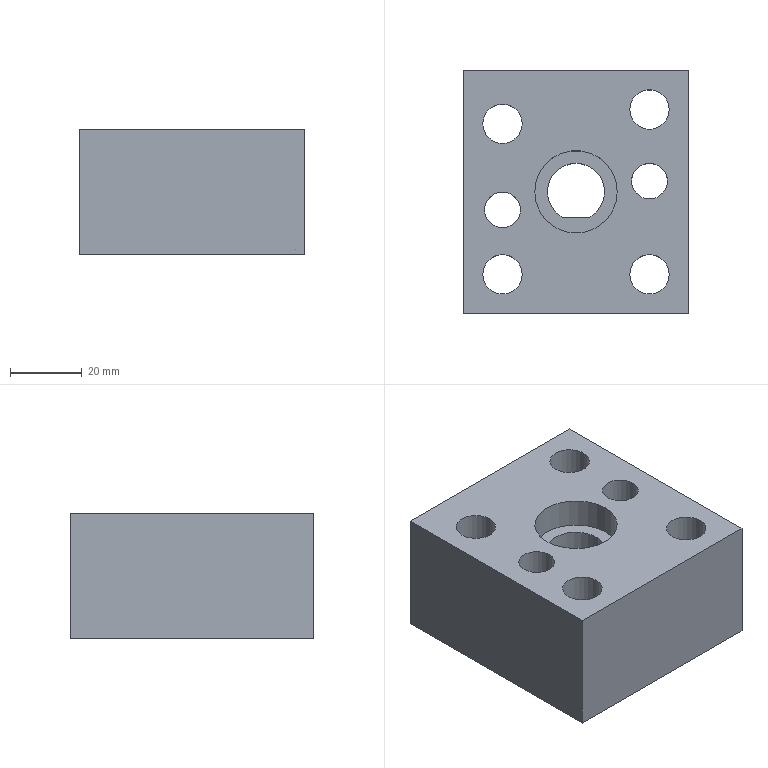Part | NX | features solid 2 | 1 solid | 28 faces | box 63 x 68 x 35 mm | volume 115819 mm3 | plane 14 | cylinder 14 | commonest cylinder face diameters 11 x6 17 x4 10 x2 16 x1 23 x1
STEP:
#1=CARTESIAN_POINT('',(1369.579,-146.904,15.));
#2=VERTEX_POINT('',#1);
#3=CARTESIAN_POINT('',(1364.579,-146.904,15.));
#4=DIRECTION('',(0.,0.,1.));
#5=DIRECTION('',(1.,0.,0.));
#6=AXIS2_PLACEMENT_3D('',#3,#4,#5);
#7=CIRCLE('',#6,5.);
#8=EDGE_CURVE('',#2,#2,#7,.T.);
#9=ORIENTED_EDGE('',*,*,#8,.T.);
#10=EDGE_LOOP('',(#9));
#11=FACE_BOUND('',#10,.T.);
#12=CARTESIAN_POINT('',(1370.079,-146.904,15.));
#13=VERTEX_POINT('',#12);
#14=CARTESIAN_POINT('',(1364.579,-146.904,15.));
#15=DIRECTION('',(0.,0.,1.));
#16=DIRECTION('',(1.,0.,0.));
#17=AXIS2_PLACEMENT_3D('',#14,#15,#16);
#18=CIRCLE('',#17,5.5);
#19=EDGE_CURVE('',#13,#13,#18,.T.);
#20=ORIENTED_EDGE('',*,*,#19,.F.);
#21=EDGE_LOOP('',(#20));
#22=FACE_BOUND('',#21,.T.);
#23=CARTESIAN_POINT('',(1363.394,-137.78,15.));
#24=DIRECTION('',(0.,0.,1.));
#25=DIRECTION('',(1.,0.,0.));
#26=AXIS2_PLACEMENT_3D('',#23,#24,#25);
#27=PLANE('',#26);
#28=ADVANCED_FACE('',(#11,#22),#27,.F.);
#29=CARTESIAN_POINT('',(1369.579,-146.904,40.));
#30=VERTEX_POINT('',#29);
#31=CARTESIAN_POINT('',(1364.579,-146.904,40.));
#32=DIRECTION('',(0.,0.,1.));
#33=DIRECTION('',(1.,0.,0.));
#34=AXIS2_PLACEMENT_3D('',#31,#32,#33);
#35=CIRCLE('',#34,5.);
#36=EDGE_CURVE('',#30,#30,#35,.T.);
#37=ORIENTED_EDGE('',*,*,#36,.T.);
#38=EDGE_LOOP('',(#37));
#39=FACE_BOUND('',#38,.T.);
#40=ORIENTED_EDGE('',*,*,#8,.F.);
#41=EDGE_LOOP('',(#40));
#42=FACE_BOUND('',#41,.T.);
#43=CARTESIAN_POINT('',(1364.579,-146.904,40.));
#44=DIRECTION('',(0.,0.,1.));
#45=DIRECTION('',(1.,0.,0.));
#46=AXIS2_PLACEMENT_3D('',#43,#44,#45);
#47=CYLINDRICAL_SURFACE('',#46,5.);
#48=ADVANCED_FACE('',(#39,#42),#47,.F.);
#49=CARTESIAN_POINT('',(1370.079,-146.904,5.));
#50=VERTEX_POINT('',#49);
#51=CARTESIAN_POINT('',(1364.579,-146.904,5.));
#52=DIRECTION('',(0.,0.,1.));
#53=DIRECTION('',(1.,0.,0.));
#54=AXIS2_PLACEMENT_3D('',#51,#52,#53);
#55=CIRCLE('',#54,5.5);
#56=EDGE_CURVE('',#50,#50,#55,.F.);
#57=ORIENTED_EDGE('',*,*,#56,.T.);
#58=EDGE_LOOP('',(#57));
#59=FACE_BOUND('',#58,.T.);
#60=ORIENTED_EDGE('',*,*,#19,.T.);
#61=EDGE_LOOP('',(#60));
#62=FACE_BOUND('',#61,.T.);
#63=CARTESIAN_POINT('',(1364.579,-146.904,5.));
#64=DIRECTION('',(0.,0.,1.));
#65=DIRECTION('',(1.,0.,0.));
#66=AXIS2_PLACEMENT_3D('',#63,#64,#65);
#67=CYLINDRICAL_SURFACE('',#66,5.5);
#68=ADVANCED_FACE('',(#59,#62),#67,.F.);
#69=CARTESIAN_POINT('',(1400.079,-164.904,17.));
#70=VERTEX_POINT('',#69);
#71=CARTESIAN_POINT('',(1405.579,-164.904,17.));
#72=DIRECTION('',(0.,0.,1.));
#73=DIRECTION('',(-1.,0.,0.));
#74=AXIS2_PLACEMENT_3D('',#71,#72,#73);
#75=CIRCLE('',#74,5.5);
#76=EDGE_CURVE('',#70,#70,#75,.T.);
#77=ORIENTED_EDGE('',*,*,#76,.T.);
#78=EDGE_LOOP('',(#77));
#79=FACE_BOUND('',#78,.T.);
#80=CARTESIAN_POINT('',(1397.079,-164.904,17.));
#81=VERTEX_POINT('',#80);
#82=CARTESIAN_POINT('',(1405.579,-164.904,17.));
#83=DIRECTION('',(0.,0.,1.));
#84=DIRECTION('',(-1.,0.,0.));
#85=AXIS2_PLACEMENT_3D('',#82,#83,#84);
#86=CIRCLE('',#85,8.5);
#87=EDGE_CURVE('',#81,#81,#86,.T.);
#88=ORIENTED_EDGE('',*,*,#87,.F.);
#89=EDGE_LOOP('',(#88));
#90=FACE_BOUND('',#89,.T.);
#91=CARTESIAN_POINT('',(1405.574,-163.238,17.));
#92=DIRECTION('',(0.,0.,1.));
#93=DIRECTION('',(-1.,0.,0.));
#94=AXIS2_PLACEMENT_3D('',#91,#92,#93);
#95=PLANE('',#94);
#96=ADVANCED_FACE('',(#79,#90),#95,.F.);
#97=CARTESIAN_POINT('',(1370.079,-164.904,17.));
#98=VERTEX_POINT('',#97);
#99=CARTESIAN_POINT('',(1364.579,-164.904,17.));
#100=DIRECTION('',(0.,0.,-1.));
#101=DIRECTION('',(1.,0.,0.));
#102=AXIS2_PLACEMENT_3D('',#99,#100,#101);
#103=CIRCLE('',#102,5.5);
#104=EDGE_CURVE('',#98,#98,#103,.F.);
#105=ORIENTED_EDGE('',*,*,#104,.T.);
#106=EDGE_LOOP('',(#105));
#107=FACE_BOUND('',#106,.T.);
#108=CARTESIAN_POINT('',(1373.079,-164.904,17.));
#109=VERTEX_POINT('',#108);
#110=CARTESIAN_POINT('',(1364.579,-164.904,17.));
#111=DIRECTION('',(0.,0.,-1.));
#112=DIRECTION('',(1.,0.,0.));
#113=AXIS2_PLACEMENT_3D('',#110,#111,#112);
#114=CIRCLE('',#113,8.5);
#115=EDGE_CURVE('',#109,#109,#114,.F.);
#116=ORIENTED_EDGE('',*,*,#115,.F.);
#117=EDGE_LOOP('',(#116));
#118=FACE_BOUND('',#117,.T.);
#119=CARTESIAN_POINT('',(1364.583,-163.238,17.));
#120=DIRECTION('',(0.,0.,1.));
#121=DIRECTION('',(1.,0.,0.));
#122=AXIS2_PLACEMENT_3D('',#119,#120,#121);
#123=PLANE('',#122);
#124=ADVANCED_FACE('',(#107,#118),#123,.F.);
#125=CARTESIAN_POINT('',(1416.579,-107.904,5.));
#126=VERTEX_POINT('',#125);
#127=CARTESIAN_POINT('',(1416.579,-175.904,5.));
#128=VERTEX_POINT('',#127);
#129=CARTESIAN_POINT('',(1416.579,-141.904,5.));
#130=DIRECTION('',(0.,-1.,0.));
#131=VECTOR('',#130,1000.);
#132=LINE('',#129,#131);
#133=EDGE_CURVE('',#126,#128,#132,.T.);
#134=ORIENTED_EDGE('',*,*,#133,.F.);
#135=CARTESIAN_POINT('',(1416.579,-107.904,40.));
#136=VERTEX_POINT('',#135);
#137=CARTESIAN_POINT('',(1416.579,-107.904,12.));
#138=DIRECTION('',(0.,0.,1.));
#139=VECTOR('',#138,1000.);
#140=LINE('',#137,#139);
#141=EDGE_CURVE('',#126,#136,#140,.T.);
#142=ORIENTED_EDGE('',*,*,#141,.T.);
#143=CARTESIAN_POINT('',(1416.579,-175.904,40.));
#144=VERTEX_POINT('',#143);
#145=CARTESIAN_POINT('',(1416.579,-141.904,40.));
#146=DIRECTION('',(0.,-1.,0.));
#147=VECTOR('',#146,1000.);
#148=LINE('',#145,#147);
#149=EDGE_CURVE('',#144,#136,#148,.F.);
#150=ORIENTED_EDGE('',*,*,#149,.F.);
#151=CARTESIAN_POINT('',(1416.579,-175.904,12.));
#152=DIRECTION('',(0.,0.,1.));
#153=VECTOR('',#152,1000.);
#154=LINE('',#151,#153);
#155=EDGE_CURVE('',#128,#144,#154,.T.);
#156=ORIENTED_EDGE('',*,*,#155,.F.);
#157=EDGE_LOOP('',(#134,#142,#150,#156));
#158=FACE_BOUND('',#157,.T.);
#159=CARTESIAN_POINT('',(1416.579,-141.904,12.));
#160=DIRECTION('',(1.,0.,0.));
#161=DIRECTION('',(0.,0.,1.));
#162=AXIS2_PLACEMENT_3D('',#159,#160,#161);
#163=PLANE('',#162);
#164=ADVANCED_FACE('',(#158),#163,.T.);
#165=CARTESIAN_POINT('',(1353.579,-107.904,40.));
#166=VERTEX_POINT('',#165);
#167=CARTESIAN_POINT('',(1353.579,-175.904,40.));
#168=VERTEX_POINT('',#167);
#169=CARTESIAN_POINT('',(1353.579,-141.904,40.));
#170=DIRECTION('',(0.,1.,0.));
#171=VECTOR('',#170,1000.);
#172=LINE('',#169,#171);
#173=EDGE_CURVE('',#166,#168,#172,.F.);
#174=ORIENTED_EDGE('',*,*,#173,.F.);
#175=CARTESIAN_POINT('',(1353.579,-107.904,5.));
#176=VERTEX_POINT('',#175);
#177=CARTESIAN_POINT('',(1353.579,-107.904,12.));
#178=DIRECTION('',(0.,0.,1.));
#179=VECTOR('',#178,1000.);
#180=LINE('',#177,#179);
#181=EDGE_CURVE('',#176,#166,#180,.T.);
#182=ORIENTED_EDGE('',*,*,#181,.F.);
#183=CARTESIAN_POINT('',(1353.579,-175.904,5.));
#184=VERTEX_POINT('',#183);
#185=CARTESIAN_POINT('',(1353.579,-141.904,5.));
#186=DIRECTION('',(0.,1.,0.));
#187=VECTOR('',#186,1000.);
#188=LINE('',#185,#187);
#189=EDGE_CURVE('',#184,#176,#188,.T.);
#190=ORIENTED_EDGE('',*,*,#189,.F.);
#191=CARTESIAN_POINT('',(1353.579,-175.904,12.));
#192=DIRECTION('',(0.,0.,1.));
#193=VECTOR('',#192,1000.);
#194=LINE('',#191,#193);
#195=EDGE_CURVE('',#184,#168,#194,.T.);
#196=ORIENTED_EDGE('',*,*,#195,.T.);
#197=EDGE_LOOP('',(#174,#182,#190,#196));
#198=FACE_BOUND('',#197,.T.);
#199=CARTESIAN_POINT('',(1353.579,-141.904,12.));
#200=DIRECTION('',(-1.,0.,0.));
#201=DIRECTION('',(0.,0.,-1.));
#202=AXIS2_PLACEMENT_3D('',#199,#200,#201);
#203=PLANE('',#202);
#204=ADVANCED_FACE('',(#198),#203,.T.);
#205=ORIENTED_EDGE('',*,*,#195,.F.);
#206=CARTESIAN_POINT('',(1385.079,-175.904,5.));
#207=DIRECTION('',(-1.,0.,0.));
#208=VECTOR('',#207,1000.);
#209=LINE('',#206,#208);
#210=EDGE_CURVE('',#128,#184,#209,.T.);
#211=ORIENTED_EDGE('',*,*,#210,.F.);
#212=ORIENTED_EDGE('',*,*,#155,.T.);
#213=CARTESIAN_POINT('',(1385.079,-175.904,40.));
#214=DIRECTION('',(-1.,0.,0.));
#215=VECTOR('',#214,1000.);
#216=LINE('',#213,#215);
#217=EDGE_CURVE('',#168,#144,#216,.F.);
#218=ORIENTED_EDGE('',*,*,#217,.F.);
#219=EDGE_LOOP('',(#205,#211,#212,#218));
#220=FACE_BOUND('',#219,.T.);
#221=CARTESIAN_POINT('',(1385.079,-175.904,12.));
#222=DIRECTION('',(0.,-1.,0.));
#223=DIRECTION('',(0.,0.,-1.));
#224=AXIS2_PLACEMENT_3D('',#221,#222,#223);
#225=PLANE('',#224);
#226=ADVANCED_FACE('',(#220),#225,.T.);
#227=CARTESIAN_POINT('',(1400.079,-164.904,40.));
#228=VERTEX_POINT('',#227);
#229=CARTESIAN_POINT('',(1405.579,-164.904,40.));
#230=DIRECTION('',(0.,0.,1.));
#231=DIRECTION('',(-1.,0.,0.));
#232=AXIS2_PLACEMENT_3D('',#229,#230,#231);
#233=CIRCLE('',#232,5.5);
#234=EDGE_CURVE('',#228,#228,#233,.T.);
#235=ORIENTED_EDGE('',*,*,#234,.T.);
#236=EDGE_LOOP('',(#235));
#237=FACE_BOUND('',#236,.T.);
#238=ORIENTED_EDGE('',*,*,#76,.F.);
#239=EDGE_LOOP('',(#238));
#240=FACE_BOUND('',#239,.T.);
#241=CARTESIAN_POINT('',(1405.579,-164.904,40.));
#242=DIRECTION('',(0.,0.,1.));
#243=DIRECTION('',(-1.,0.,0.));
#244=AXIS2_PLACEMENT_3D('',#241,#242,#243);
#245=CYLINDRICAL_SURFACE('',#244,5.5);
#246=ADVANCED_FACE('',(#237,#240),#245,.F.);
#247=CARTESIAN_POINT('',(1370.079,-164.904,40.));
#248=VERTEX_POINT('',#247);
#249=CARTESIAN_POINT('',(1364.579,-164.904,40.));
#250=DIRECTION('',(0.,0.,-1.));
#251=DIRECTION('',(1.,0.,0.));
#252=AXIS2_PLACEMENT_3D('',#249,#250,#251);
#253=CIRCLE('',#252,5.5);
#254=EDGE_CURVE('',#248,#248,#253,.F.);
#255=ORIENTED_EDGE('',*,*,#254,.T.);
#256=EDGE_LOOP('',(#255));
#257=FACE_BOUND('',#256,.T.);
#258=ORIENTED_EDGE('',*,*,#104,.F.);
#259=EDGE_LOOP('',(#258));
#260=FACE_BOUND('',#259,.T.);
#261=CARTESIAN_POINT('',(1364.579,-164.904,40.));
#262=DIRECTION('',(0.,0.,1.));
#263=DIRECTION('',(1.,0.,0.));
#264=AXIS2_PLACEMENT_3D('',#261,#262,#263);
#265=CYLINDRICAL_SURFACE('',#264,5.5);
#266=ADVANCED_FACE('',(#257,#260),#265,.F.);
#267=ORIENTED_EDGE('',*,*,#36,.F.);
#268=EDGE_LOOP('',(#267));
#269=FACE_BOUND('',#268,.T.);
#270=ORIENTED_EDGE('',*,*,#149,.T.);
#271=CARTESIAN_POINT('',(1385.079,-107.904,40.));
#272=DIRECTION('',(1.,0.,0.));
#273=VECTOR('',#272,1000.);
#274=LINE('',#271,#273);
#275=EDGE_CURVE('',#136,#166,#274,.F.);
#276=ORIENTED_EDGE('',*,*,#275,.T.);
#277=ORIENTED_EDGE('',*,*,#173,.T.);
#278=ORIENTED_EDGE('',*,*,#217,.T.);
#279=EDGE_LOOP('',(#270,#276,#277,#278));
#280=FACE_BOUND('',#279,.T.);
#281=CARTESIAN_POINT('',(1373.579,-141.904,40.));
#282=VERTEX_POINT('',#281);
#283=CARTESIAN_POINT('',(1385.079,-141.904,40.));
#284=DIRECTION('',(0.,0.,-1.));
#285=DIRECTION('',(-1.,0.,0.));
#286=AXIS2_PLACEMENT_3D('',#283,#284,#285);
#287=CIRCLE('',#286,11.5);
#288=EDGE_CURVE('',#282,#282,#287,.F.);
#289=ORIENTED_EDGE('',*,*,#288,.F.);
#290=EDGE_LOOP('',(#289));
#291=FACE_BOUND('',#290,.T.);
#292=ORIENTED_EDGE('',*,*,#254,.F.);
#293=EDGE_LOOP('',(#292));
#294=FACE_BOUND('',#293,.T.);
#295=ORIENTED_EDGE('',*,*,#234,.F.);
#296=EDGE_LOOP('',(#295));
#297=FACE_BOUND('',#296,.T.);
#298=CARTESIAN_POINT('',(1400.079,-118.904,40.));
#299=VERTEX_POINT('',#298);
#300=CARTESIAN_POINT('',(1405.579,-118.904,40.));
#301=DIRECTION('',(0.,0.,-1.));
#302=DIRECTION('',(-1.,0.,0.));
#303=AXIS2_PLACEMENT_3D('',#300,#301,#302);
#304=CIRCLE('',#303,5.5);
#305=EDGE_CURVE('',#299,#299,#304,.T.);
#306=ORIENTED_EDGE('',*,*,#305,.T.);
#307=EDGE_LOOP('',(#306));
#308=FACE_BOUND('',#307,.T.);
#309=CARTESIAN_POINT('',(1370.079,-122.904,40.));
#310=VERTEX_POINT('',#309);
#311=CARTESIAN_POINT('',(1364.579,-122.904,40.));
#312=DIRECTION('',(0.,0.,1.));
#313=DIRECTION('',(1.,0.,0.));
#314=AXIS2_PLACEMENT_3D('',#311,#312,#313);
#315=CIRCLE('',#314,5.5);
#316=EDGE_CURVE('',#310,#310,#315,.T.);
#317=ORIENTED_EDGE('',*,*,#316,.F.);
#318=EDGE_LOOP('',(#317));
#319=FACE_BOUND('',#318,.T.);
#320=CARTESIAN_POINT('',(1400.579,-138.904,40.));
#321=VERTEX_POINT('',#320);
#322=CARTESIAN_POINT('',(1405.579,-138.904,40.));
#323=DIRECTION('',(0.,0.,-1.));
#324=DIRECTION('',(-1.,0.,0.));
#325=AXIS2_PLACEMENT_3D('',#322,#323,#324);
#326=CIRCLE('',#325,5.);
#327=EDGE_CURVE('',#321,#321,#326,.T.);
#328=ORIENTED_EDGE('',*,*,#327,.T.);
#329=EDGE_LOOP('',(#328));
#330=FACE_BOUND('',#329,.T.);
#331=CARTESIAN_POINT('',(2186.158,-0.000000688,40.));
#332=DIRECTION('',(0.,0.,-1.));
#333=DIRECTION('',(1.,0.,0.));
#334=AXIS2_PLACEMENT_3D('',#331,#332,#333);
#335=PLANE('',#334);
#336=ADVANCED_FACE('',(#269,#280,#291,#294,#297,#308,#319,#330),#335,.F.);
#337=ORIENTED_EDGE('',*,*,#87,.T.);
#338=EDGE_LOOP('',(#337));
#339=FACE_BOUND('',#338,.T.);
#340=CARTESIAN_POINT('',(1397.079,-164.904,5.));
#341=VERTEX_POINT('',#340);
#342=CARTESIAN_POINT('',(1405.579,-164.904,5.));
#343=DIRECTION('',(0.,0.,1.));
#344=DIRECTION('',(-1.,0.,0.));
#345=AXIS2_PLACEMENT_3D('',#342,#343,#344);
#346=CIRCLE('',#345,8.5);
#347=EDGE_CURVE('',#341,#341,#346,.F.);
#348=ORIENTED_EDGE('',*,*,#347,.T.);
#349=EDGE_LOOP('',(#348));
#350=FACE_BOUND('',#349,.T.);
#351=CARTESIAN_POINT('',(1405.579,-164.904,5.));
#352=DIRECTION('',(0.,0.,1.));
#353=DIRECTION('',(-1.,0.,0.));
#354=AXIS2_PLACEMENT_3D('',#351,#352,#353);
#355=CYLINDRICAL_SURFACE('',#354,8.5);
#356=ADVANCED_FACE('',(#339,#350),#355,.F.);
#357=ORIENTED_EDGE('',*,*,#115,.T.);
#358=EDGE_LOOP('',(#357));
#359=FACE_BOUND('',#358,.T.);
#360=CARTESIAN_POINT('',(1373.079,-164.904,5.));
#361=VERTEX_POINT('',#360);
#362=CARTESIAN_POINT('',(1364.579,-164.904,5.));
#363=DIRECTION('',(0.,0.,-1.));
#364=DIRECTION('',(1.,0.,0.));
#365=AXIS2_PLACEMENT_3D('',#362,#363,#364);
#366=CIRCLE('',#365,8.5);
#367=EDGE_CURVE('',#361,#361,#366,.T.);
#368=ORIENTED_EDGE('',*,*,#367,.T.);
#369=EDGE_LOOP('',(#368));
#370=FACE_BOUND('',#369,.T.);
#371=CARTESIAN_POINT('',(1364.579,-164.904,5.));
#372=DIRECTION('',(0.,0.,1.));
#373=DIRECTION('',(1.,0.,0.));
#374=AXIS2_PLACEMENT_3D('',#371,#372,#373);
#375=CYLINDRICAL_SURFACE('',#374,8.5);
#376=ADVANCED_FACE('',(#359,#370),#375,.F.);
#377=CARTESIAN_POINT('',(1388.952,-148.904,5.));
#378=VERTEX_POINT('',#377);
#379=CARTESIAN_POINT('',(1381.206,-148.904,5.));
#380=VERTEX_POINT('',#379);
#381=CARTESIAN_POINT('',(1385.079,-148.904,5.));
#382=DIRECTION('',(-1.,0.,0.));
#383=VECTOR('',#382,1000.);
#384=LINE('',#381,#383);
#385=EDGE_CURVE('',#378,#380,#384,.T.);
#386=ORIENTED_EDGE('',*,*,#385,.F.);
#387=CARTESIAN_POINT('',(1385.079,-141.904,5.));
#388=DIRECTION('',(0.,0.,-1.));
#389=DIRECTION('',(-1.,0.,0.));
#390=AXIS2_PLACEMENT_3D('',#387,#388,#389);
#391=CIRCLE('',#390,8.);
#392=EDGE_CURVE('',#378,#380,#391,.F.);
#393=ORIENTED_EDGE('',*,*,#392,.T.);
#394=EDGE_LOOP('',(#386,#393));
#395=FACE_BOUND('',#394,.T.);
#396=CARTESIAN_POINT('',(1385.079,-107.904,5.));
#397=DIRECTION('',(1.,0.,0.));
#398=VECTOR('',#397,1000.);
#399=LINE('',#396,#398);
#400=EDGE_CURVE('',#176,#126,#399,.T.);
#401=ORIENTED_EDGE('',*,*,#400,.T.);
#402=ORIENTED_EDGE('',*,*,#133,.T.);
#403=ORIENTED_EDGE('',*,*,#210,.T.);
#404=ORIENTED_EDGE('',*,*,#189,.T.);
#405=EDGE_LOOP('',(#401,#402,#403,#404));
#406=FACE_BOUND('',#405,.T.);
#407=ORIENTED_EDGE('',*,*,#56,.F.);
#408=EDGE_LOOP('',(#407));
#409=FACE_BOUND('',#408,.T.);
#410=ORIENTED_EDGE('',*,*,#367,.F.);
#411=EDGE_LOOP('',(#410));
#412=FACE_BOUND('',#411,.T.);
#413=ORIENTED_EDGE('',*,*,#347,.F.);
#414=EDGE_LOOP('',(#413));
#415=FACE_BOUND('',#414,.T.);
#416=CARTESIAN_POINT('',(1397.079,-118.904,5.));
#417=VERTEX_POINT('',#416);
#418=CARTESIAN_POINT('',(1405.579,-118.904,5.));
#419=DIRECTION('',(0.,0.,-1.));
#420=DIRECTION('',(-1.,0.,0.));
#421=AXIS2_PLACEMENT_3D('',#418,#419,#420);
#422=CIRCLE('',#421,8.5);
#423=EDGE_CURVE('',#417,#417,#422,.T.);
#424=ORIENTED_EDGE('',*,*,#423,.F.);
#425=EDGE_LOOP('',(#424));
#426=FACE_BOUND('',#425,.T.);
#427=CARTESIAN_POINT('',(1373.079,-122.904,5.));
#428=VERTEX_POINT('',#427);
#429=CARTESIAN_POINT('',(1364.579,-122.904,5.));
#430=DIRECTION('',(0.,0.,1.));
#431=DIRECTION('',(1.,0.,0.));
#432=AXIS2_PLACEMENT_3D('',#429,#430,#431);
#433=CIRCLE('',#432,8.5);
#434=EDGE_CURVE('',#428,#428,#433,.F.);
#435=ORIENTED_EDGE('',*,*,#434,.F.);
#436=EDGE_LOOP('',(#435));
#437=FACE_BOUND('',#436,.T.);
#438=CARTESIAN_POINT('',(1400.079,-138.904,5.));
#439=VERTEX_POINT('',#438);
#440=CARTESIAN_POINT('',(1405.579,-138.904,5.));
#441=DIRECTION('',(0.,0.,-1.));
#442=DIRECTION('',(-1.,0.,0.));
#443=AXIS2_PLACEMENT_3D('',#440,#441,#442);
#444=CIRCLE('',#443,5.5);
#445=EDGE_CURVE('',#439,#439,#444,.T.);
#446=ORIENTED_EDGE('',*,*,#445,.F.);
#447=EDGE_LOOP('',(#446));
#448=FACE_BOUND('',#447,.T.);
#449=CARTESIAN_POINT('',(1385.079,-141.904,5.));
#450=DIRECTION('',(0.,0.,-1.));
#451=DIRECTION('',(1.,0.,0.));
#452=AXIS2_PLACEMENT_3D('',#449,#450,#451);
#453=PLANE('',#452);
#454=ADVANCED_FACE('',(#395,#406,#409,#412,#415,#426,#437,#448),#453,.T.);
#455=CARTESIAN_POINT('',(1373.579,-141.904,31.8));
#456=VERTEX_POINT('',#455);
#457=CARTESIAN_POINT('',(1385.079,-141.904,31.8));
#458=DIRECTION('',(0.,0.,-1.));
#459=DIRECTION('',(-1.,0.,0.));
#460=AXIS2_PLACEMENT_3D('',#457,#458,#459);
#461=CIRCLE('',#460,11.5);
#462=EDGE_CURVE('',#456,#456,#461,.T.);
#463=ORIENTED_EDGE('',*,*,#462,.T.);
#464=EDGE_LOOP('',(#463));
#465=FACE_BOUND('',#464,.T.);
#466=ORIENTED_EDGE('',*,*,#288,.T.);
#467=EDGE_LOOP('',(#466));
#468=FACE_BOUND('',#467,.T.);
#469=CARTESIAN_POINT('',(1385.079,-141.904,40.));
#470=DIRECTION('',(0.,0.,-1.));
#471=DIRECTION('',(1.,0.,0.));
#472=AXIS2_PLACEMENT_3D('',#469,#470,#471);
#473=CYLINDRICAL_SURFACE('',#472,11.5);
#474=ADVANCED_FACE('',(#465,#468),#473,.F.);
#475=CARTESIAN_POINT('',(1388.952,-148.904,31.8));
#476=VERTEX_POINT('',#475);
#477=CARTESIAN_POINT('',(1381.206,-148.904,31.8));
#478=VERTEX_POINT('',#477);
#479=CARTESIAN_POINT('',(1385.079,-141.904,31.8));
#480=DIRECTION('',(0.,0.,-1.));
#481=DIRECTION('',(-1.,0.,0.));
#482=AXIS2_PLACEMENT_3D('',#479,#480,#481);
#483=CIRCLE('',#482,8.);
#484=EDGE_CURVE('',#476,#478,#483,.F.);
#485=ORIENTED_EDGE('',*,*,#484,.F.);
#486=CARTESIAN_POINT('',(2087.158,-148.904,31.8));
#487=DIRECTION('',(-1.,0.,0.));
#488=VECTOR('',#487,1000.);
#489=LINE('',#486,#488);
#490=EDGE_CURVE('',#476,#478,#489,.T.);
#491=ORIENTED_EDGE('',*,*,#490,.T.);
#492=EDGE_LOOP('',(#485,#491));
#493=FACE_BOUND('',#492,.T.);
#494=ORIENTED_EDGE('',*,*,#462,.F.);
#495=EDGE_LOOP('',(#494));
#496=FACE_BOUND('',#495,.T.);
#497=CARTESIAN_POINT('',(2087.158,-0.000000688,31.8));
#498=DIRECTION('',(0.,0.,-1.));
#499=DIRECTION('',(1.,0.,0.));
#500=AXIS2_PLACEMENT_3D('',#497,#498,#499);
#501=PLANE('',#500);
#502=ADVANCED_FACE('',(#493,#496),#501,.F.);
#503=ORIENTED_EDGE('',*,*,#385,.T.);
#504=CARTESIAN_POINT('',(1381.206,-148.904,40.));
#505=DIRECTION('',(0.,0.,-1.));
#506=VECTOR('',#505,1000.);
#507=LINE('',#504,#506);
#508=EDGE_CURVE('',#380,#478,#507,.F.);
#509=ORIENTED_EDGE('',*,*,#508,.T.);
#510=ORIENTED_EDGE('',*,*,#490,.F.);
#511=CARTESIAN_POINT('',(1388.952,-148.904,40.));
#512=DIRECTION('',(0.,0.,-1.));
#513=VECTOR('',#512,1000.);
#514=LINE('',#511,#513);
#515=EDGE_CURVE('',#476,#378,#514,.T.);
#516=ORIENTED_EDGE('',*,*,#515,.T.);
#517=EDGE_LOOP('',(#503,#509,#510,#516));
#518=FACE_BOUND('',#517,.T.);
#519=CARTESIAN_POINT('',(1385.079,-148.904,14.995));
#520=DIRECTION('',(0.,-1.,0.));
#521=DIRECTION('',(0.,0.,-1.));
#522=AXIS2_PLACEMENT_3D('',#519,#520,#521);
#523=PLANE('',#522);
#524=ADVANCED_FACE('',(#518),#523,.F.);
#525=CARTESIAN_POINT('',(1400.579,-138.904,15.));
#526=VERTEX_POINT('',#525);
#527=CARTESIAN_POINT('',(1405.579,-138.904,15.));
#528=DIRECTION('',(0.,0.,-1.));
#529=DIRECTION('',(-1.,0.,0.));
#530=AXIS2_PLACEMENT_3D('',#527,#528,#529);
#531=CIRCLE('',#530,5.);
#532=EDGE_CURVE('',#526,#526,#531,.F.);
#533=ORIENTED_EDGE('',*,*,#532,.T.);
#534=EDGE_LOOP('',(#533));
#535=FACE_BOUND('',#534,.T.);
#536=CARTESIAN_POINT('',(1400.079,-138.904,15.));
#537=VERTEX_POINT('',#536);
#538=CARTESIAN_POINT('',(1405.579,-138.904,15.));
#539=DIRECTION('',(0.,0.,-1.));
#540=DIRECTION('',(-1.,0.,0.));
#541=AXIS2_PLACEMENT_3D('',#538,#539,#540);
#542=CIRCLE('',#541,5.5);
#543=EDGE_CURVE('',#537,#537,#542,.F.);
#544=ORIENTED_EDGE('',*,*,#543,.F.);
#545=EDGE_LOOP('',(#544));
#546=FACE_BOUND('',#545,.T.);
#547=CARTESIAN_POINT('',(1406.763,-137.78,15.));
#548=DIRECTION('',(0.,0.,1.));
#549=DIRECTION('',(-1.,0.,0.));
#550=AXIS2_PLACEMENT_3D('',#547,#548,#549);
#551=PLANE('',#550);
#552=ADVANCED_FACE('',(#535,#546),#551,.F.);
#553=CARTESIAN_POINT('',(1370.079,-122.904,17.));
#554=VERTEX_POINT('',#553);
#555=CARTESIAN_POINT('',(1364.579,-122.904,17.));
#556=DIRECTION('',(0.,0.,1.));
#557=DIRECTION('',(1.,0.,0.));
#558=AXIS2_PLACEMENT_3D('',#555,#556,#557);
#559=CIRCLE('',#558,5.5);
#560=EDGE_CURVE('',#554,#554,#559,.T.);
#561=ORIENTED_EDGE('',*,*,#560,.T.);
#562=EDGE_LOOP('',(#561));
#563=FACE_BOUND('',#562,.T.);
#564=CARTESIAN_POINT('',(1373.079,-122.904,17.));
#565=VERTEX_POINT('',#564);
#566=CARTESIAN_POINT('',(1364.579,-122.904,17.));
#567=DIRECTION('',(0.,0.,1.));
#568=DIRECTION('',(1.,0.,0.));
#569=AXIS2_PLACEMENT_3D('',#566,#567,#568);
#570=CIRCLE('',#569,8.5);
#571=EDGE_CURVE('',#565,#565,#570,.T.);
#572=ORIENTED_EDGE('',*,*,#571,.F.);
#573=EDGE_LOOP('',(#572));
#574=FACE_BOUND('',#573,.T.);
#575=CARTESIAN_POINT('',(1364.583,-124.57,17.));
#576=DIRECTION('',(0.,0.,1.));
#577=DIRECTION('',(1.,0.,0.));
#578=AXIS2_PLACEMENT_3D('',#575,#576,#577);
#579=PLANE('',#578);
#580=ADVANCED_FACE('',(#563,#574),#579,.F.);
#581=CARTESIAN_POINT('',(1400.079,-118.904,17.));
#582=VERTEX_POINT('',#581);
#583=CARTESIAN_POINT('',(1405.579,-118.904,17.));
#584=DIRECTION('',(0.,0.,-1.));
#585=DIRECTION('',(-1.,0.,0.));
#586=AXIS2_PLACEMENT_3D('',#583,#584,#585);
#587=CIRCLE('',#586,5.5);
#588=EDGE_CURVE('',#582,#582,#587,.F.);
#589=ORIENTED_EDGE('',*,*,#588,.T.);
#590=EDGE_LOOP('',(#589));
#591=FACE_BOUND('',#590,.T.);
#592=CARTESIAN_POINT('',(1397.079,-118.904,17.));
#593=VERTEX_POINT('',#592);
#594=CARTESIAN_POINT('',(1405.579,-118.904,17.));
#595=DIRECTION('',(0.,0.,-1.));
#596=DIRECTION('',(-1.,0.,0.));
#597=AXIS2_PLACEMENT_3D('',#594,#595,#596);
#598=CIRCLE('',#597,8.5);
#599=EDGE_CURVE('',#593,#593,#598,.F.);
#600=ORIENTED_EDGE('',*,*,#599,.F.);
#601=EDGE_LOOP('',(#600));
#602=FACE_BOUND('',#601,.T.);
#603=CARTESIAN_POINT('',(1405.574,-120.57,17.));
#604=DIRECTION('',(0.,0.,1.));
#605=DIRECTION('',(-1.,0.,0.));
#606=AXIS2_PLACEMENT_3D('',#603,#604,#605);
#607=PLANE('',#606);
#608=ADVANCED_FACE('',(#591,#602),#607,.F.);
#609=ORIENTED_EDGE('',*,*,#327,.F.);
#610=EDGE_LOOP('',(#609));
#611=FACE_BOUND('',#610,.T.);
#612=ORIENTED_EDGE('',*,*,#532,.F.);
#613=EDGE_LOOP('',(#612));
#614=FACE_BOUND('',#613,.T.);
#615=CARTESIAN_POINT('',(1405.579,-138.904,40.));
#616=DIRECTION('',(0.,0.,1.));
#617=DIRECTION('',(-1.,0.,0.));
#618=AXIS2_PLACEMENT_3D('',#615,#616,#617);
#619=CYLINDRICAL_SURFACE('',#618,5.);
#620=ADVANCED_FACE('',(#611,#614),#619,.F.);
#621=ORIENTED_EDGE('',*,*,#316,.T.);
#622=EDGE_LOOP('',(#621));
#623=FACE_BOUND('',#622,.T.);
#624=ORIENTED_EDGE('',*,*,#560,.F.);
#625=EDGE_LOOP('',(#624));
#626=FACE_BOUND('',#625,.T.);
#627=CARTESIAN_POINT('',(1364.579,-122.904,40.));
#628=DIRECTION('',(0.,0.,1.));
#629=DIRECTION('',(1.,0.,0.));
#630=AXIS2_PLACEMENT_3D('',#627,#628,#629);
#631=CYLINDRICAL_SURFACE('',#630,5.5);
#632=ADVANCED_FACE('',(#623,#626),#631,.F.);
#633=ORIENTED_EDGE('',*,*,#305,.F.);
#634=EDGE_LOOP('',(#633));
#635=FACE_BOUND('',#634,.T.);
#636=ORIENTED_EDGE('',*,*,#588,.F.);
#637=EDGE_LOOP('',(#636));
#638=FACE_BOUND('',#637,.T.);
#639=CARTESIAN_POINT('',(1405.579,-118.904,40.));
#640=DIRECTION('',(0.,0.,1.));
#641=DIRECTION('',(-1.,0.,0.));
#642=AXIS2_PLACEMENT_3D('',#639,#640,#641);
#643=CYLINDRICAL_SURFACE('',#642,5.5);
#644=ADVANCED_FACE('',(#635,#638),#643,.F.);
#645=ORIENTED_EDGE('',*,*,#141,.F.);
#646=ORIENTED_EDGE('',*,*,#400,.F.);
#647=ORIENTED_EDGE('',*,*,#181,.T.);
#648=ORIENTED_EDGE('',*,*,#275,.F.);
#649=EDGE_LOOP('',(#645,#646,#647,#648));
#650=FACE_BOUND('',#649,.T.);
#651=CARTESIAN_POINT('',(1385.079,-107.904,12.));
#652=DIRECTION('',(0.,1.,0.));
#653=DIRECTION('',(0.,0.,1.));
#654=AXIS2_PLACEMENT_3D('',#651,#652,#653);
#655=PLANE('',#654);
#656=ADVANCED_FACE('',(#650),#655,.T.);
#657=ORIENTED_EDGE('',*,*,#543,.T.);
#658=EDGE_LOOP('',(#657));
#659=FACE_BOUND('',#658,.T.);
#660=ORIENTED_EDGE('',*,*,#445,.T.);
#661=EDGE_LOOP('',(#660));
#662=FACE_BOUND('',#661,.T.);
#663=CARTESIAN_POINT('',(1405.579,-138.904,5.));
#664=DIRECTION('',(0.,0.,1.));
#665=DIRECTION('',(-1.,0.,0.));
#666=AXIS2_PLACEMENT_3D('',#663,#664,#665);
#667=CYLINDRICAL_SURFACE('',#666,5.5);
#668=ADVANCED_FACE('',(#659,#662),#667,.F.);
#669=ORIENTED_EDGE('',*,*,#571,.T.);
#670=EDGE_LOOP('',(#669));
#671=FACE_BOUND('',#670,.T.);
#672=ORIENTED_EDGE('',*,*,#434,.T.);
#673=EDGE_LOOP('',(#672));
#674=FACE_BOUND('',#673,.T.);
#675=CARTESIAN_POINT('',(1364.579,-122.904,5.));
#676=DIRECTION('',(0.,0.,1.));
#677=DIRECTION('',(1.,0.,0.));
#678=AXIS2_PLACEMENT_3D('',#675,#676,#677);
#679=CYLINDRICAL_SURFACE('',#678,8.5);
#680=ADVANCED_FACE('',(#671,#674),#679,.F.);
#681=ORIENTED_EDGE('',*,*,#599,.T.);
#682=EDGE_LOOP('',(#681));
#683=FACE_BOUND('',#682,.T.);
#684=ORIENTED_EDGE('',*,*,#423,.T.);
#685=EDGE_LOOP('',(#684));
#686=FACE_BOUND('',#685,.T.);
#687=CARTESIAN_POINT('',(1405.579,-118.904,5.));
#688=DIRECTION('',(0.,0.,1.));
#689=DIRECTION('',(-1.,0.,0.));
#690=AXIS2_PLACEMENT_3D('',#687,#688,#689);
#691=CYLINDRICAL_SURFACE('',#690,8.5);
#692=ADVANCED_FACE('',(#683,#686),#691,.F.);
#693=ORIENTED_EDGE('',*,*,#508,.F.);
#694=ORIENTED_EDGE('',*,*,#392,.F.);
#695=ORIENTED_EDGE('',*,*,#515,.F.);
#696=ORIENTED_EDGE('',*,*,#484,.T.);
#697=EDGE_LOOP('',(#693,#694,#695,#696));
#698=FACE_BOUND('',#697,.T.);
#699=CARTESIAN_POINT('',(1385.079,-141.904,40.));
#700=DIRECTION('',(0.,0.,-1.));
#701=DIRECTION('',(1.,0.,0.));
#702=AXIS2_PLACEMENT_3D('',#699,#700,#701);
#703=CYLINDRICAL_SURFACE('',#702,8.);
#704=ADVANCED_FACE('',(#698),#703,.F.);
#705=CLOSED_SHELL('',(#28,#48,#68,#96,#124,#164,#204,#226,#246,#266,#336,#356,#376,#454,#474,#502,#524,#552,#580,#608,#620,#632,#644,#656,#668,#680,#692,#704));
#706=MANIFOLD_SOLID_BREP('',#705);
#707=(LENGTH_UNIT()NAMED_UNIT(*)SI_UNIT(.MILLI.,.METRE.));
#708=UNCERTAINTY_MEASURE_WITH_UNIT(LENGTH_MEASURE(0.00001),#707,'','');
#709=(NAMED_UNIT(*)PLANE_ANGLE_UNIT()SI_UNIT($,.RADIAN.));
#710=(NAMED_UNIT(*)SI_UNIT($,.STERADIAN.)SOLID_ANGLE_UNIT());
#711=(GEOMETRIC_REPRESENTATION_CONTEXT(3)GLOBAL_UNCERTAINTY_ASSIGNED_CONTEXT((#708))GLOBAL_UNIT_ASSIGNED_CONTEXT((#707,#709,#710))REPRESENTATION_CONTEXT('',''));
#712=ADVANCED_BREP_SHAPE_REPRESENTATION('',(#706),#711);